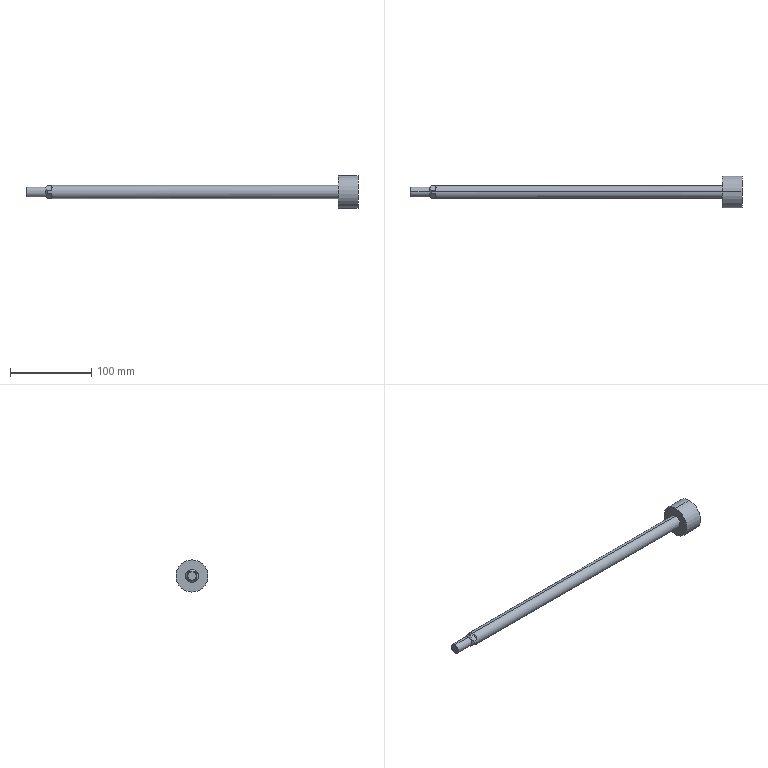Part | SolidWorks | features BaseBody 1 | 1 solid | 21 faces | box 407.5 x 39.5 x 39.5 mm | volume 104182 mm3 | plane 11 | cylinder 6 | cone 4 | commonest cylinder face diameters 12 x2 16 x2 39.5 x2
STEP:
#1=CARTESIAN_POINT('',(334.5,0.,-19.75));
#2=VERTEX_POINT('',#1);
#3=CARTESIAN_POINT('',(358.5,0.,-19.75));
#4=VERTEX_POINT('',#3);
#5=CARTESIAN_POINT('',(358.5,0.,-19.75));
#6=DIRECTION('',(1.,0.,0.));
#7=VECTOR('',#6,1000.);
#8=LINE('',#5,#7);
#9=EDGE_CURVE('',#2,#4,#8,.T.);
#10=ORIENTED_EDGE('',*,*,#9,.F.);
#11=CARTESIAN_POINT('',(334.5,0.,19.75));
#12=VERTEX_POINT('',#11);
#13=CARTESIAN_POINT('',(334.5,0.,0.));
#14=DIRECTION('',(1.,0.,0.));
#15=DIRECTION('',(0.,0.,-1.));
#16=AXIS2_PLACEMENT_3D('',#13,#14,#15);
#17=CIRCLE('',#16,19.75);
#18=EDGE_CURVE('',#2,#12,#17,.T.);
#19=ORIENTED_EDGE('',*,*,#18,.T.);
#20=CARTESIAN_POINT('',(358.5,-0.000000023,19.75));
#21=VERTEX_POINT('',#20);
#22=CARTESIAN_POINT('',(358.5,0.,19.75));
#23=DIRECTION('',(1.,0.,0.));
#24=VECTOR('',#23,1000.);
#25=LINE('',#22,#24);
#26=EDGE_CURVE('',#12,#21,#25,.T.);
#27=ORIENTED_EDGE('',*,*,#26,.T.);
#28=CARTESIAN_POINT('',(358.5,0.,0.));
#29=DIRECTION('',(1.,0.,0.));
#30=DIRECTION('',(0.,-0.000000001,1.));
#31=AXIS2_PLACEMENT_3D('',#28,#29,#30);
#32=CIRCLE('',#31,19.75);
#33=EDGE_CURVE('',#4,#21,#32,.T.);
#34=ORIENTED_EDGE('',*,*,#33,.F.);
#35=EDGE_LOOP('',(#10,#19,#27,#34));
#36=FACE_OUTER_BOUND('',#35,.T.);
#37=CARTESIAN_POINT('',(358.5,0.,0.));
#38=DIRECTION('',(1.,0.,0.));
#39=DIRECTION('',(0.,0.,1.));
#40=AXIS2_PLACEMENT_3D('',#37,#38,#39);
#41=CYLINDRICAL_SURFACE('',#40,19.75);
#42=ADVANCED_FACE('',(#36),#41,.T.);
#43=CARTESIAN_POINT('',(-48.233,0.,-6.));
#44=VERTEX_POINT('',#43);
#45=CARTESIAN_POINT('',(-25.,0.,-6.));
#46=VERTEX_POINT('',#45);
#47=CARTESIAN_POINT('',(358.5,0.,-6.));
#48=DIRECTION('',(1.,0.,0.));
#49=VECTOR('',#48,1000.);
#50=LINE('',#47,#49);
#51=EDGE_CURVE('',#44,#46,#50,.T.);
#52=ORIENTED_EDGE('',*,*,#51,.F.);
#53=CARTESIAN_POINT('',(-48.233,0.,6.));
#54=VERTEX_POINT('',#53);
#55=CARTESIAN_POINT('',(-48.233,0.,0.));
#56=DIRECTION('',(1.,0.,0.));
#57=DIRECTION('',(0.,0.,-1.));
#58=AXIS2_PLACEMENT_3D('',#55,#56,#57);
#59=CIRCLE('',#58,6.);
#60=EDGE_CURVE('',#44,#54,#59,.T.);
#61=ORIENTED_EDGE('',*,*,#60,.T.);
#62=CARTESIAN_POINT('',(-25.,0.,6.));
#63=VERTEX_POINT('',#62);
#64=CARTESIAN_POINT('',(358.5,0.,6.));
#65=DIRECTION('',(1.,0.,0.));
#66=VECTOR('',#65,1000.);
#67=LINE('',#64,#66);
#68=EDGE_CURVE('',#54,#63,#67,.T.);
#69=ORIENTED_EDGE('',*,*,#68,.T.);
#70=CARTESIAN_POINT('',(-25.,0.,0.));
#71=DIRECTION('',(1.,0.,0.));
#72=DIRECTION('',(0.,0.,1.));
#73=AXIS2_PLACEMENT_3D('',#70,#71,#72);
#74=CIRCLE('',#73,6.);
#75=EDGE_CURVE('',#46,#63,#74,.T.);
#76=ORIENTED_EDGE('',*,*,#75,.F.);
#77=EDGE_LOOP('',(#52,#61,#69,#76));
#78=FACE_OUTER_BOUND('',#77,.T.);
#79=CARTESIAN_POINT('',(358.5,0.,0.));
#80=DIRECTION('',(1.,0.,0.));
#81=DIRECTION('',(0.,0.,1.));
#82=AXIS2_PLACEMENT_3D('',#79,#80,#81);
#83=CYLINDRICAL_SURFACE('',#82,6.);
#84=ADVANCED_FACE('',(#78),#83,.T.);
#85=CARTESIAN_POINT('',(-49.,0.,-5.233));
#86=VERTEX_POINT('',#85);
#87=CARTESIAN_POINT('',(-48.233,0.,-6.));
#88=DIRECTION('',(0.7071,0.,-0.7071));
#89=VECTOR('',#88,1000.);
#90=LINE('',#87,#89);
#91=EDGE_CURVE('',#86,#44,#90,.T.);
#92=ORIENTED_EDGE('',*,*,#91,.F.);
#93=CARTESIAN_POINT('',(-49.,0.,5.233));
#94=VERTEX_POINT('',#93);
#95=CARTESIAN_POINT('',(-49.,0.,0.));
#96=DIRECTION('',(1.,0.,0.));
#97=DIRECTION('',(0.,0.,-1.));
#98=AXIS2_PLACEMENT_3D('',#95,#96,#97);
#99=CIRCLE('',#98,5.233);
#100=EDGE_CURVE('',#86,#94,#99,.T.);
#101=ORIENTED_EDGE('',*,*,#100,.T.);
#102=CARTESIAN_POINT('',(-48.233,0.,6.));
#103=DIRECTION('',(0.7071,0.,0.7071));
#104=VECTOR('',#103,1000.);
#105=LINE('',#102,#104);
#106=EDGE_CURVE('',#94,#54,#105,.T.);
#107=ORIENTED_EDGE('',*,*,#106,.T.);
#108=ORIENTED_EDGE('',*,*,#60,.F.);
#109=EDGE_LOOP('',(#92,#101,#107,#108));
#110=FACE_OUTER_BOUND('',#109,.T.);
#111=CARTESIAN_POINT('',(-48.233,0.,0.));
#112=DIRECTION('',(1.,0.,0.));
#113=DIRECTION('',(0.,0.,1.));
#114=AXIS2_PLACEMENT_3D('',#111,#112,#113);
#115=CONICAL_SURFACE('',#114,6.,0.7854);
#116=ADVANCED_FACE('',(#110),#115,.T.);
#117=CARTESIAN_POINT('',(-23.,0.,-8.));
#118=VERTEX_POINT('',#117);
#119=CARTESIAN_POINT('',(334.5,0.,-8.));
#120=VERTEX_POINT('',#119);
#121=CARTESIAN_POINT('',(358.5,0.,-8.));
#122=DIRECTION('',(1.,0.,0.));
#123=VECTOR('',#122,1000.);
#124=LINE('',#121,#123);
#125=EDGE_CURVE('',#118,#120,#124,.T.);
#126=ORIENTED_EDGE('',*,*,#125,.F.);
#127=CARTESIAN_POINT('',(-23.,2.211,-7.688));
#128=VERTEX_POINT('',#127);
#129=CARTESIAN_POINT('',(-23.,0.,0.));
#130=DIRECTION('',(1.,0.,0.));
#131=DIRECTION('',(0.,0.2764,-0.961));
#132=AXIS2_PLACEMENT_3D('',#129,#130,#131);
#133=CIRCLE('',#132,8.);
#134=EDGE_CURVE('',#118,#128,#133,.T.);
#135=ORIENTED_EDGE('',*,*,#134,.T.);
#136=CARTESIAN_POINT('',(-18.,2.211,-7.688));
#137=VERTEX_POINT('',#136);
#138=CARTESIAN_POINT('',(-18.,2.211,-7.688));
#139=DIRECTION('',(-1.,0.,0.));
#140=VECTOR('',#139,1000.);
#141=LINE('',#138,#140);
#142=EDGE_CURVE('',#137,#128,#141,.T.);
#143=ORIENTED_EDGE('',*,*,#142,.F.);
#144=CARTESIAN_POINT('',(-18.,7.688,-2.211));
#145=VERTEX_POINT('',#144);
#146=CARTESIAN_POINT('',(-18.,7.688,-2.211));
#147=CARTESIAN_POINT('',(-17.344,7.314,-3.513));
#148=CARTESIAN_POINT('',(-17.,6.615,-4.699));
#149=CARTESIAN_POINT('',(-17.,4.699,-6.615));
#150=CARTESIAN_POINT('',(-17.344,3.513,-7.314));
#151=CARTESIAN_POINT('',(-18.,2.211,-7.688));
#152=B_SPLINE_CURVE_WITH_KNOTS('',3,(#146,#147,#148,#149,#150,#151),.UNSPECIFIED.,.F.,.F.,(4,2,4),(0.,0.5,1.),.UNSPECIFIED.);
#153=EDGE_CURVE('',#145,#137,#152,.T.);
#154=ORIENTED_EDGE('',*,*,#153,.F.);
#155=CARTESIAN_POINT('',(-23.,7.688,-2.211));
#156=VERTEX_POINT('',#155);
#157=CARTESIAN_POINT('',(-23.,7.688,-2.211));
#158=DIRECTION('',(1.,0.,0.));
#159=VECTOR('',#158,1000.);
#160=LINE('',#157,#159);
#161=EDGE_CURVE('',#156,#145,#160,.T.);
#162=ORIENTED_EDGE('',*,*,#161,.F.);
#163=CARTESIAN_POINT('',(-23.,7.688,2.211));
#164=VERTEX_POINT('',#163);
#165=CARTESIAN_POINT('',(-23.,0.,0.));
#166=DIRECTION('',(1.,0.,0.));
#167=DIRECTION('',(0.,0.961,0.2764));
#168=AXIS2_PLACEMENT_3D('',#165,#166,#167);
#169=CIRCLE('',#168,8.);
#170=EDGE_CURVE('',#156,#164,#169,.T.);
#171=ORIENTED_EDGE('',*,*,#170,.T.);
#172=CARTESIAN_POINT('',(-18.,7.688,2.211));
#173=VERTEX_POINT('',#172);
#174=CARTESIAN_POINT('',(-18.,7.688,2.211));
#175=DIRECTION('',(-1.,0.,0.));
#176=VECTOR('',#175,1000.);
#177=LINE('',#174,#176);
#178=EDGE_CURVE('',#173,#164,#177,.T.);
#179=ORIENTED_EDGE('',*,*,#178,.F.);
#180=CARTESIAN_POINT('',(-18.,2.211,7.688));
#181=VERTEX_POINT('',#180);
#182=CARTESIAN_POINT('',(-18.,2.211,7.688));
#183=CARTESIAN_POINT('',(-17.835,2.539,7.594));
#184=CARTESIAN_POINT('',(-17.69,2.858,7.48));
#185=CARTESIAN_POINT('',(-17.44,3.478,7.213));
#186=CARTESIAN_POINT('',(-17.335,3.781,7.058));
#187=CARTESIAN_POINT('',(-17.167,4.365,6.713));
#188=CARTESIAN_POINT('',(-17.072,4.783,6.429));
#189=CARTESIAN_POINT('',(-17.025,5.172,6.106));
#190=CARTESIAN_POINT('',(-17.004,5.425,5.883));
#191=CARTESIAN_POINT('',(-16.999,5.546,5.768));
#192=CARTESIAN_POINT('',(-17.,5.909,5.404));
#193=CARTESIAN_POINT('',(-17.034,6.246,5.02));
#194=CARTESIAN_POINT('',(-17.13,6.594,4.535));
#195=CARTESIAN_POINT('',(-17.193,6.757,4.284));
#196=CARTESIAN_POINT('',(-17.222,6.824,4.175));
#197=CARTESIAN_POINT('',(-17.243,6.869,4.101));
#198=CARTESIAN_POINT('',(-17.254,6.891,4.063));
#199=CARTESIAN_POINT('',(-17.433,7.246,3.455));
#200=CARTESIAN_POINT('',(-17.679,7.505,2.849));
#201=CARTESIAN_POINT('',(-18.,7.688,2.211));
#202=B_SPLINE_CURVE_WITH_KNOTS('',3,(#182,#183,#184,#185,#186,#187,#188,#189,#190,#191,#192,#193,#194,#195,#196,#197,#198,#199,#200,#201),.UNSPECIFIED.,.F.,.F.,(4,2,2,1,2,2,1,1,1,2,2,4),(0.,0.125,0.25,0.375,0.4375,0.5,0.625,0.6875,0.7187,0.7344,0.75,1.),.UNSPECIFIED.);
#203=EDGE_CURVE('',#181,#173,#202,.T.);
#204=ORIENTED_EDGE('',*,*,#203,.F.);
#205=CARTESIAN_POINT('',(-23.,2.211,7.688));
#206=VERTEX_POINT('',#205);
#207=CARTESIAN_POINT('',(-23.,2.211,7.688));
#208=DIRECTION('',(1.,0.,0.));
#209=VECTOR('',#208,1000.);
#210=LINE('',#207,#209);
#211=EDGE_CURVE('',#206,#181,#210,.T.);
#212=ORIENTED_EDGE('',*,*,#211,.F.);
#213=CARTESIAN_POINT('',(-23.,0.,8.));
#214=VERTEX_POINT('',#213);
#215=CARTESIAN_POINT('',(-23.,0.,0.));
#216=DIRECTION('',(1.,0.,0.));
#217=DIRECTION('',(0.,-0.2764,0.961));
#218=AXIS2_PLACEMENT_3D('',#215,#216,#217);
#219=CIRCLE('',#218,8.);
#220=EDGE_CURVE('',#206,#214,#219,.T.);
#221=ORIENTED_EDGE('',*,*,#220,.T.);
#222=CARTESIAN_POINT('',(334.5,0.,8.));
#223=VERTEX_POINT('',#222);
#224=CARTESIAN_POINT('',(358.5,0.,8.));
#225=DIRECTION('',(1.,0.,0.));
#226=VECTOR('',#225,1000.);
#227=LINE('',#224,#226);
#228=EDGE_CURVE('',#214,#223,#227,.T.);
#229=ORIENTED_EDGE('',*,*,#228,.T.);
#230=CARTESIAN_POINT('',(334.5,0.,0.));
#231=DIRECTION('',(1.,0.,0.));
#232=DIRECTION('',(0.,0.,1.));
#233=AXIS2_PLACEMENT_3D('',#230,#231,#232);
#234=CIRCLE('',#233,8.);
#235=EDGE_CURVE('',#120,#223,#234,.T.);
#236=ORIENTED_EDGE('',*,*,#235,.F.);
#237=EDGE_LOOP('',(#126,#135,#143,#154,#162,#171,#179,#204,#212,#221,#229,#236));
#238=FACE_OUTER_BOUND('',#237,.T.);
#239=CARTESIAN_POINT('',(358.5,0.,0.));
#240=DIRECTION('',(1.,0.,0.));
#241=DIRECTION('',(0.,0.,1.));
#242=AXIS2_PLACEMENT_3D('',#239,#240,#241);
#243=CYLINDRICAL_SURFACE('',#242,8.);
#244=ADVANCED_FACE('',(#238),#243,.T.);
#245=CARTESIAN_POINT('',(-23.,0.,-8.));
#246=DIRECTION('',(0.7071,0.,-0.7071));
#247=VECTOR('',#246,1000.);
#248=LINE('',#245,#247);
#249=EDGE_CURVE('',#46,#118,#248,.T.);
#250=ORIENTED_EDGE('',*,*,#249,.F.);
#251=ORIENTED_EDGE('',*,*,#75,.T.);
#252=CARTESIAN_POINT('',(-23.,0.,8.));
#253=DIRECTION('',(0.7071,0.,0.7071));
#254=VECTOR('',#253,1000.);
#255=LINE('',#252,#254);
#256=EDGE_CURVE('',#63,#214,#255,.T.);
#257=ORIENTED_EDGE('',*,*,#256,.T.);
#258=ORIENTED_EDGE('',*,*,#220,.F.);
#259=CARTESIAN_POINT('',(-23.,7.688,2.211));
#260=CARTESIAN_POINT('',(-23.157,7.459,2.44));
#261=CARTESIAN_POINT('',(-23.364,7.123,2.776));
#262=CARTESIAN_POINT('',(-23.556,6.746,3.153));
#263=CARTESIAN_POINT('',(-23.639,6.561,3.338));
#264=CARTESIAN_POINT('',(-23.678,6.47,3.43));
#265=CARTESIAN_POINT('',(-23.696,6.424,3.476));
#266=CARTESIAN_POINT('',(-23.704,6.404,3.495));
#267=CARTESIAN_POINT('',(-23.709,6.391,3.508));
#268=CARTESIAN_POINT('',(-23.712,6.386,3.514));
#269=CARTESIAN_POINT('',(-23.805,6.147,3.753));
#270=CARTESIAN_POINT('',(-23.909,5.802,4.098));
#271=CARTESIAN_POINT('',(-23.973,5.405,4.495));
#272=CARTESIAN_POINT('',(-23.991,5.207,4.692));
#273=CARTESIAN_POINT('',(-23.995,5.123,4.776));
#274=CARTESIAN_POINT('',(-23.998,5.067,4.833));
#275=CARTESIAN_POINT('',(-23.998,5.04,4.859));
#276=CARTESIAN_POINT('',(-24.003,4.777,5.123));
#277=CARTESIAN_POINT('',(-23.974,4.422,5.477));
#278=CARTESIAN_POINT('',(-23.876,4.002,5.897));
#279=CARTESIAN_POINT('',(-23.811,3.791,6.109));
#280=CARTESIAN_POINT('',(-23.775,3.685,6.215));
#281=CARTESIAN_POINT('',(-23.756,3.632,6.268));
#282=CARTESIAN_POINT('',(-23.748,3.609,6.291));
#283=CARTESIAN_POINT('',(-23.742,3.594,6.306));
#284=CARTESIAN_POINT('',(-23.739,3.585,6.314));
#285=CARTESIAN_POINT('',(-23.573,3.145,6.754));
#286=CARTESIAN_POINT('',(-23.327,2.689,7.21));
#287=CARTESIAN_POINT('',(-23.,2.211,7.688));
#288=B_SPLINE_CURVE_WITH_KNOTS('',3,(#259,#260,#261,#262,#263,#264,#265,#266,#267,#268,#269,#270,#271,#272,#273,#274,#275,#276,#277,#278,#279,#280,#281,#282,#283,#284,#285,#286,#287),.UNSPECIFIED.,.F.,.F.,(4,1,1,1,1,1,2,2,1,1,1,2,2,1,1,1,1,1,2,2,4),(0.,0.125,0.1875,0.2188,0.2344,0.2422,0.2461,0.25,0.375,0.4375,0.4687,0.4844,0.5,0.625,0.6875,0.7187,0.7344,0.7422,0.7461,0.75,1.),.UNSPECIFIED.);
#289=EDGE_CURVE('',#164,#206,#288,.T.);
#290=ORIENTED_EDGE('',*,*,#289,.F.);
#291=ORIENTED_EDGE('',*,*,#170,.F.);
#292=CARTESIAN_POINT('',(-23.,2.211,-7.688));
#293=CARTESIAN_POINT('',(-23.157,2.44,-7.459));
#294=CARTESIAN_POINT('',(-23.364,2.776,-7.123));
#295=CARTESIAN_POINT('',(-23.556,3.153,-6.746));
#296=CARTESIAN_POINT('',(-23.639,3.338,-6.561));
#297=CARTESIAN_POINT('',(-23.678,3.43,-6.47));
#298=CARTESIAN_POINT('',(-23.696,3.476,-6.424));
#299=CARTESIAN_POINT('',(-23.704,3.495,-6.404));
#300=CARTESIAN_POINT('',(-23.709,3.508,-6.391));
#301=CARTESIAN_POINT('',(-23.712,3.514,-6.386));
#302=CARTESIAN_POINT('',(-23.805,3.753,-6.147));
#303=CARTESIAN_POINT('',(-23.909,4.098,-5.802));
#304=CARTESIAN_POINT('',(-23.973,4.495,-5.405));
#305=CARTESIAN_POINT('',(-23.991,4.692,-5.207));
#306=CARTESIAN_POINT('',(-23.995,4.776,-5.123));
#307=CARTESIAN_POINT('',(-23.998,4.833,-5.067));
#308=CARTESIAN_POINT('',(-23.998,4.859,-5.04));
#309=CARTESIAN_POINT('',(-24.003,5.123,-4.777));
#310=CARTESIAN_POINT('',(-23.974,5.477,-4.422));
#311=CARTESIAN_POINT('',(-23.876,5.897,-4.002));
#312=CARTESIAN_POINT('',(-23.811,6.109,-3.791));
#313=CARTESIAN_POINT('',(-23.775,6.215,-3.685));
#314=CARTESIAN_POINT('',(-23.756,6.268,-3.632));
#315=CARTESIAN_POINT('',(-23.748,6.291,-3.609));
#316=CARTESIAN_POINT('',(-23.742,6.306,-3.594));
#317=CARTESIAN_POINT('',(-23.739,6.314,-3.585));
#318=CARTESIAN_POINT('',(-23.573,6.754,-3.145));
#319=CARTESIAN_POINT('',(-23.327,7.21,-2.689));
#320=CARTESIAN_POINT('',(-23.,7.688,-2.211));
#321=B_SPLINE_CURVE_WITH_KNOTS('',3,(#292,#293,#294,#295,#296,#297,#298,#299,#300,#301,#302,#303,#304,#305,#306,#307,#308,#309,#310,#311,#312,#313,#314,#315,#316,#317,#318,#319,#320),.UNSPECIFIED.,.F.,.F.,(4,1,1,1,1,1,2,2,1,1,1,2,2,1,1,1,1,1,2,2,4),(0.,0.125,0.1875,0.2188,0.2344,0.2422,0.2461,0.25,0.375,0.4375,0.4688,0.4844,0.5,0.625,0.6875,0.7188,0.7344,0.7422,0.7461,0.75,1.),.UNSPECIFIED.);
#322=EDGE_CURVE('',#128,#156,#321,.T.);
#323=ORIENTED_EDGE('',*,*,#322,.F.);
#324=ORIENTED_EDGE('',*,*,#134,.F.);
#325=EDGE_LOOP('',(#250,#251,#257,#258,#290,#291,#323,#324));
#326=FACE_OUTER_BOUND('',#325,.T.);
#327=CARTESIAN_POINT('',(-23.,0.,0.));
#328=DIRECTION('',(1.,0.,0.));
#329=DIRECTION('',(0.,0.,1.));
#330=AXIS2_PLACEMENT_3D('',#327,#328,#329);
#331=CONICAL_SURFACE('',#330,8.,0.7854);
#332=ADVANCED_FACE('',(#326),#331,.T.);
#333=ORIENTED_EDGE('',*,*,#161,.T.);
#334=CARTESIAN_POINT('',(-18.,2.211,-7.688));
#335=DIRECTION('',(0.,0.7071,0.7071));
#336=VECTOR('',#335,1000.);
#337=LINE('',#334,#336);
#338=EDGE_CURVE('',#137,#145,#337,.T.);
#339=ORIENTED_EDGE('',*,*,#338,.F.);
#340=ORIENTED_EDGE('',*,*,#142,.T.);
#341=ORIENTED_EDGE('',*,*,#322,.T.);
#342=EDGE_LOOP('',(#333,#339,#340,#341));
#343=FACE_OUTER_BOUND('',#342,.T.);
#344=CARTESIAN_POINT('',(-24.151,2.211,-7.688));
#345=DIRECTION('',(0.,0.7071,-0.7071));
#346=DIRECTION('',(-1.,0.,0.));
#347=AXIS2_PLACEMENT_3D('',#344,#345,#346);
#348=PLANE('',#347);
#349=ADVANCED_FACE('',(#343),#348,.T.);
#350=ORIENTED_EDGE('',*,*,#153,.T.);
#351=ORIENTED_EDGE('',*,*,#338,.T.);
#352=EDGE_LOOP('',(#350,#351));
#353=FACE_OUTER_BOUND('',#352,.T.);
#354=CARTESIAN_POINT('',(-17.979,2.211,-7.718));
#355=DIRECTION('',(-0.7071,0.5,-0.5));
#356=DIRECTION('',(-0.5774,0.,0.8165));
#357=AXIS2_PLACEMENT_3D('',#354,#355,#356);
#358=PLANE('',#357);
#359=ADVANCED_FACE('',(#353),#358,.T.);
#360=CARTESIAN_POINT('',(-23.,-7.688,2.211));
#361=VERTEX_POINT('',#360);
#362=CARTESIAN_POINT('',(-18.,-7.688,2.211));
#363=VERTEX_POINT('',#362);
#364=CARTESIAN_POINT('',(-23.,-7.688,2.211));
#365=DIRECTION('',(1.,0.,0.));
#366=VECTOR('',#365,1000.);
#367=LINE('',#364,#366);
#368=EDGE_CURVE('',#361,#363,#367,.T.);
#369=ORIENTED_EDGE('',*,*,#368,.T.);
#370=CARTESIAN_POINT('',(-18.,-2.211,7.688));
#371=VERTEX_POINT('',#370);
#372=CARTESIAN_POINT('',(-18.,-2.211,7.688));
#373=DIRECTION('',(0.,0.7071,0.7071));
#374=VECTOR('',#373,1000.);
#375=LINE('',#372,#374);
#376=EDGE_CURVE('',#363,#371,#375,.T.);
#377=ORIENTED_EDGE('',*,*,#376,.T.);
#378=CARTESIAN_POINT('',(-23.,-2.211,7.688));
#379=VERTEX_POINT('',#378);
#380=CARTESIAN_POINT('',(-18.,-2.211,7.688));
#381=DIRECTION('',(-1.,0.,0.));
#382=VECTOR('',#381,1000.);
#383=LINE('',#380,#382);
#384=EDGE_CURVE('',#371,#379,#383,.T.);
#385=ORIENTED_EDGE('',*,*,#384,.T.);
#386=CARTESIAN_POINT('',(-23.,-2.211,7.688));
#387=CARTESIAN_POINT('',(-23.157,-2.44,7.459));
#388=CARTESIAN_POINT('',(-23.364,-2.776,7.123));
#389=CARTESIAN_POINT('',(-23.556,-3.153,6.746));
#390=CARTESIAN_POINT('',(-23.639,-3.338,6.561));
#391=CARTESIAN_POINT('',(-23.678,-3.43,6.47));
#392=CARTESIAN_POINT('',(-23.696,-3.476,6.424));
#393=CARTESIAN_POINT('',(-23.704,-3.495,6.404));
#394=CARTESIAN_POINT('',(-23.709,-3.508,6.391));
#395=CARTESIAN_POINT('',(-23.712,-3.514,6.386));
#396=CARTESIAN_POINT('',(-23.805,-3.753,6.147));
#397=CARTESIAN_POINT('',(-23.909,-4.098,5.802));
#398=CARTESIAN_POINT('',(-23.973,-4.495,5.405));
#399=CARTESIAN_POINT('',(-23.991,-4.692,5.207));
#400=CARTESIAN_POINT('',(-23.995,-4.776,5.123));
#401=CARTESIAN_POINT('',(-23.998,-4.833,5.067));
#402=CARTESIAN_POINT('',(-23.998,-4.859,5.04));
#403=CARTESIAN_POINT('',(-24.003,-5.123,4.777));
#404=CARTESIAN_POINT('',(-23.974,-5.477,4.422));
#405=CARTESIAN_POINT('',(-23.876,-5.897,4.002));
#406=CARTESIAN_POINT('',(-23.811,-6.109,3.791));
#407=CARTESIAN_POINT('',(-23.775,-6.215,3.685));
#408=CARTESIAN_POINT('',(-23.756,-6.268,3.632));
#409=CARTESIAN_POINT('',(-23.748,-6.291,3.609));
#410=CARTESIAN_POINT('',(-23.742,-6.306,3.594));
#411=CARTESIAN_POINT('',(-23.739,-6.314,3.585));
#412=CARTESIAN_POINT('',(-23.573,-6.754,3.145));
#413=CARTESIAN_POINT('',(-23.327,-7.21,2.689));
#414=CARTESIAN_POINT('',(-23.,-7.688,2.211));
#415=B_SPLINE_CURVE_WITH_KNOTS('',3,(#386,#387,#388,#389,#390,#391,#392,#393,#394,#395,#396,#397,#398,#399,#400,#401,#402,#403,#404,#405,#406,#407,#408,#409,#410,#411,#412,#413,#414),.UNSPECIFIED.,.F.,.F.,(4,1,1,1,1,1,2,2,1,1,1,2,2,1,1,1,1,1,2,2,4),(0.,0.125,0.1875,0.2187,0.2344,0.2422,0.2461,0.25,0.375,0.4375,0.4687,0.4844,0.5,0.625,0.6875,0.7188,0.7344,0.7422,0.7461,0.75,1.),.UNSPECIFIED.);
#416=EDGE_CURVE('',#379,#361,#415,.T.);
#417=ORIENTED_EDGE('',*,*,#416,.T.);
#418=EDGE_LOOP('',(#369,#377,#385,#417));
#419=FACE_OUTER_BOUND('',#418,.T.);
#420=CARTESIAN_POINT('',(-24.151,-2.211,7.688));
#421=DIRECTION('',(0.,-0.7071,0.7071));
#422=DIRECTION('',(-1.,0.,0.));
#423=AXIS2_PLACEMENT_3D('',#420,#421,#422);
#424=PLANE('',#423);
#425=ADVANCED_FACE('',(#419),#424,.T.);
#426=CARTESIAN_POINT('',(-18.,-7.688,2.211));
#427=CARTESIAN_POINT('',(-17.344,-7.314,3.513));
#428=CARTESIAN_POINT('',(-17.,-6.615,4.699));
#429=CARTESIAN_POINT('',(-17.,-4.699,6.615));
#430=CARTESIAN_POINT('',(-17.344,-3.513,7.314));
#431=CARTESIAN_POINT('',(-18.,-2.211,7.688));
#432=B_SPLINE_CURVE_WITH_KNOTS('',3,(#426,#427,#428,#429,#430,#431),.UNSPECIFIED.,.F.,.F.,(4,2,4),(0.,0.5,1.),.UNSPECIFIED.);
#433=EDGE_CURVE('',#363,#371,#432,.T.);
#434=ORIENTED_EDGE('',*,*,#433,.T.);
#435=ORIENTED_EDGE('',*,*,#376,.F.);
#436=EDGE_LOOP('',(#434,#435));
#437=FACE_OUTER_BOUND('',#436,.T.);
#438=CARTESIAN_POINT('',(-18.,-7.688,2.211));
#439=DIRECTION('',(-0.7071,-0.5,0.5));
#440=DIRECTION('',(-0.5774,0.8165,0.));
#441=AXIS2_PLACEMENT_3D('',#438,#439,#440);
#442=PLANE('',#441);
#443=ADVANCED_FACE('',(#437),#442,.T.);
#444=CARTESIAN_POINT('',(-23.,-2.211,-7.688));
#445=VERTEX_POINT('',#444);
#446=CARTESIAN_POINT('',(-18.,-2.211,-7.688));
#447=VERTEX_POINT('',#446);
#448=CARTESIAN_POINT('',(-23.,-2.211,-7.688));
#449=DIRECTION('',(1.,0.,0.));
#450=VECTOR('',#449,1000.);
#451=LINE('',#448,#450);
#452=EDGE_CURVE('',#445,#447,#451,.T.);
#453=ORIENTED_EDGE('',*,*,#452,.T.);
#454=CARTESIAN_POINT('',(-18.,-7.688,-2.211));
#455=VERTEX_POINT('',#454);
#456=CARTESIAN_POINT('',(-18.,-7.688,-2.211));
#457=DIRECTION('',(0.,0.7071,-0.7071));
#458=VECTOR('',#457,1000.);
#459=LINE('',#456,#458);
#460=EDGE_CURVE('',#455,#447,#459,.T.);
#461=ORIENTED_EDGE('',*,*,#460,.F.);
#462=CARTESIAN_POINT('',(-23.,-7.688,-2.211));
#463=VERTEX_POINT('',#462);
#464=CARTESIAN_POINT('',(-18.,-7.688,-2.211));
#465=DIRECTION('',(-1.,0.,0.));
#466=VECTOR('',#465,1000.);
#467=LINE('',#464,#466);
#468=EDGE_CURVE('',#455,#463,#467,.T.);
#469=ORIENTED_EDGE('',*,*,#468,.T.);
#470=CARTESIAN_POINT('',(-23.,-7.688,-2.211));
#471=CARTESIAN_POINT('',(-23.157,-7.459,-2.44));
#472=CARTESIAN_POINT('',(-23.364,-7.123,-2.776));
#473=CARTESIAN_POINT('',(-23.556,-6.746,-3.153));
#474=CARTESIAN_POINT('',(-23.639,-6.561,-3.338));
#475=CARTESIAN_POINT('',(-23.678,-6.47,-3.43));
#476=CARTESIAN_POINT('',(-23.696,-6.424,-3.476));
#477=CARTESIAN_POINT('',(-23.704,-6.404,-3.495));
#478=CARTESIAN_POINT('',(-23.709,-6.391,-3.508));
#479=CARTESIAN_POINT('',(-23.712,-6.386,-3.514));
#480=CARTESIAN_POINT('',(-23.805,-6.147,-3.753));
#481=CARTESIAN_POINT('',(-23.909,-5.802,-4.098));
#482=CARTESIAN_POINT('',(-23.973,-5.405,-4.495));
#483=CARTESIAN_POINT('',(-23.991,-5.207,-4.692));
#484=CARTESIAN_POINT('',(-23.995,-5.123,-4.776));
#485=CARTESIAN_POINT('',(-23.998,-5.067,-4.833));
#486=CARTESIAN_POINT('',(-23.998,-5.04,-4.859));
#487=CARTESIAN_POINT('',(-24.003,-4.777,-5.123));
#488=CARTESIAN_POINT('',(-23.974,-4.422,-5.477));
#489=CARTESIAN_POINT('',(-23.876,-4.002,-5.897));
#490=CARTESIAN_POINT('',(-23.811,-3.791,-6.109));
#491=CARTESIAN_POINT('',(-23.775,-3.685,-6.215));
#492=CARTESIAN_POINT('',(-23.756,-3.632,-6.268));
#493=CARTESIAN_POINT('',(-23.748,-3.609,-6.291));
#494=CARTESIAN_POINT('',(-23.742,-3.594,-6.306));
#495=CARTESIAN_POINT('',(-23.739,-3.585,-6.314));
#496=CARTESIAN_POINT('',(-23.573,-3.145,-6.754));
#497=CARTESIAN_POINT('',(-23.327,-2.689,-7.21));
#498=CARTESIAN_POINT('',(-23.,-2.211,-7.688));
#499=B_SPLINE_CURVE_WITH_KNOTS('',3,(#470,#471,#472,#473,#474,#475,#476,#477,#478,#479,#480,#481,#482,#483,#484,#485,#486,#487,#488,#489,#490,#491,#492,#493,#494,#495,#496,#497,#498),.UNSPECIFIED.,.F.,.F.,(4,1,1,1,1,1,2,2,1,1,1,2,2,1,1,1,1,1,2,2,4),(0.,0.125,0.1875,0.2188,0.2344,0.2422,0.2461,0.25,0.375,0.4375,0.4688,0.4844,0.5,0.625,0.6875,0.7188,0.7344,0.7422,0.7461,0.75,1.),.UNSPECIFIED.);
#500=EDGE_CURVE('',#463,#445,#499,.T.);
#501=ORIENTED_EDGE('',*,*,#500,.T.);
#502=EDGE_LOOP('',(#453,#461,#469,#501));
#503=FACE_OUTER_BOUND('',#502,.T.);
#504=CARTESIAN_POINT('',(-24.151,-7.688,-2.211));
#505=DIRECTION('',(0.,-0.7071,-0.7071));
#506=DIRECTION('',(0.,-0.7071,0.7071));
#507=AXIS2_PLACEMENT_3D('',#504,#505,#506);
#508=PLANE('',#507);
#509=ADVANCED_FACE('',(#503),#508,.T.);
#510=CARTESIAN_POINT('',(-18.,-2.211,-7.688));
#511=CARTESIAN_POINT('',(-17.835,-2.539,-7.594));
#512=CARTESIAN_POINT('',(-17.69,-2.858,-7.48));
#513=CARTESIAN_POINT('',(-17.44,-3.478,-7.213));
#514=CARTESIAN_POINT('',(-17.335,-3.781,-7.058));
#515=CARTESIAN_POINT('',(-17.167,-4.365,-6.713));
#516=CARTESIAN_POINT('',(-17.072,-4.783,-6.429));
#517=CARTESIAN_POINT('',(-17.025,-5.172,-6.106));
#518=CARTESIAN_POINT('',(-17.004,-5.425,-5.883));
#519=CARTESIAN_POINT('',(-16.999,-5.546,-5.768));
#520=CARTESIAN_POINT('',(-17.,-5.909,-5.404));
#521=CARTESIAN_POINT('',(-17.034,-6.246,-5.02));
#522=CARTESIAN_POINT('',(-17.13,-6.594,-4.535));
#523=CARTESIAN_POINT('',(-17.193,-6.757,-4.284));
#524=CARTESIAN_POINT('',(-17.222,-6.824,-4.175));
#525=CARTESIAN_POINT('',(-17.243,-6.869,-4.101));
#526=CARTESIAN_POINT('',(-17.254,-6.891,-4.063));
#527=CARTESIAN_POINT('',(-17.433,-7.246,-3.455));
#528=CARTESIAN_POINT('',(-17.679,-7.505,-2.849));
#529=CARTESIAN_POINT('',(-18.,-7.688,-2.211));
#530=B_SPLINE_CURVE_WITH_KNOTS('',3,(#510,#511,#512,#513,#514,#515,#516,#517,#518,#519,#520,#521,#522,#523,#524,#525,#526,#527,#528,#529),.UNSPECIFIED.,.F.,.F.,(4,2,2,1,2,2,1,1,1,2,2,4),(0.,0.125,0.25,0.375,0.4375,0.5,0.625,0.6875,0.7188,0.7344,0.75,1.),.UNSPECIFIED.);
#531=EDGE_CURVE('',#447,#455,#530,.T.);
#532=ORIENTED_EDGE('',*,*,#531,.T.);
#533=ORIENTED_EDGE('',*,*,#460,.T.);
#534=EDGE_LOOP('',(#532,#533));
#535=FACE_OUTER_BOUND('',#534,.T.);
#536=CARTESIAN_POINT('',(-15.386,-7.688,-5.907));
#537=DIRECTION('',(-0.7071,-0.5,-0.5));
#538=DIRECTION('',(-0.5774,0.8165,0.));
#539=AXIS2_PLACEMENT_3D('',#536,#537,#538);
#540=PLANE('',#539);
#541=ADVANCED_FACE('',(#535),#540,.T.);
#542=ORIENTED_EDGE('',*,*,#211,.T.);
#543=CARTESIAN_POINT('',(-18.,7.688,2.211));
#544=DIRECTION('',(0.,0.7071,-0.7071));
#545=VECTOR('',#544,1000.);
#546=LINE('',#543,#545);
#547=EDGE_CURVE('',#181,#173,#546,.T.);
#548=ORIENTED_EDGE('',*,*,#547,.T.);
#549=ORIENTED_EDGE('',*,*,#178,.T.);
#550=ORIENTED_EDGE('',*,*,#289,.T.);
#551=EDGE_LOOP('',(#542,#548,#549,#550));
#552=FACE_OUTER_BOUND('',#551,.T.);
#553=CARTESIAN_POINT('',(-24.151,7.688,2.211));
#554=DIRECTION('',(0.,0.7071,0.7071));
#555=DIRECTION('',(1.,0.,0.));
#556=AXIS2_PLACEMENT_3D('',#553,#554,#555);
#557=PLANE('',#556);
#558=ADVANCED_FACE('',(#552),#557,.T.);
#559=ORIENTED_EDGE('',*,*,#203,.T.);
#560=ORIENTED_EDGE('',*,*,#547,.F.);
#561=EDGE_LOOP('',(#559,#560));
#562=FACE_OUTER_BOUND('',#561,.T.);
#563=CARTESIAN_POINT('',(-20.582,2.211,4.037));
#564=DIRECTION('',(-0.7071,0.5,0.5));
#565=DIRECTION('',(0.5774,0.,0.8165));
#566=AXIS2_PLACEMENT_3D('',#563,#564,#565);
#567=PLANE('',#566);
#568=ADVANCED_FACE('',(#562),#567,.T.);
#569=CARTESIAN_POINT('',(358.5,0.,0.));
#570=DIRECTION('',(1.,0.,0.));
#571=DIRECTION('',(0.,-0.000000001,1.));
#572=AXIS2_PLACEMENT_3D('',#569,#570,#571);
#573=CIRCLE('',#572,19.75);
#574=EDGE_CURVE('',#21,#4,#573,.T.);
#575=ORIENTED_EDGE('',*,*,#574,.T.);
#576=ORIENTED_EDGE('',*,*,#33,.T.);
#577=EDGE_LOOP('',(#575,#576));
#578=FACE_OUTER_BOUND('',#577,.T.);
#579=CARTESIAN_POINT('',(358.5,-20.117,-19.75));
#580=DIRECTION('',(1.,0.,0.));
#581=DIRECTION('',(0.,1.,0.));
#582=AXIS2_PLACEMENT_3D('',#579,#580,#581);
#583=PLANE('',#582);
#584=ADVANCED_FACE('',(#578),#583,.T.);
#585=CARTESIAN_POINT('',(334.5,0.,0.));
#586=DIRECTION('',(1.,0.,0.));
#587=DIRECTION('',(0.,0.,1.));
#588=AXIS2_PLACEMENT_3D('',#585,#586,#587);
#589=CIRCLE('',#588,8.);
#590=EDGE_CURVE('',#223,#120,#589,.T.);
#591=ORIENTED_EDGE('',*,*,#590,.T.);
#592=ORIENTED_EDGE('',*,*,#235,.T.);
#593=EDGE_LOOP('',(#591,#592));
#594=FACE_BOUND('',#593,.T.);
#595=CARTESIAN_POINT('',(334.5,0.,0.));
#596=DIRECTION('',(1.,0.,0.));
#597=DIRECTION('',(0.,0.,-1.));
#598=AXIS2_PLACEMENT_3D('',#595,#596,#597);
#599=CIRCLE('',#598,19.75);
#600=EDGE_CURVE('',#12,#2,#599,.T.);
#601=ORIENTED_EDGE('',*,*,#600,.F.);
#602=ORIENTED_EDGE('',*,*,#18,.F.);
#603=EDGE_LOOP('',(#601,#602));
#604=FACE_OUTER_BOUND('',#603,.T.);
#605=CARTESIAN_POINT('',(334.5,-20.117,19.75));
#606=DIRECTION('',(-1.,0.,0.));
#607=DIRECTION('',(0.,0.,1.));
#608=AXIS2_PLACEMENT_3D('',#605,#606,#607);
#609=PLANE('',#608);
#610=ADVANCED_FACE('',(#594,#604),#609,.T.);
#611=CARTESIAN_POINT('',(-49.,0.,0.));
#612=DIRECTION('',(1.,0.,0.));
#613=DIRECTION('',(0.,0.,-1.));
#614=AXIS2_PLACEMENT_3D('',#611,#612,#613);
#615=CIRCLE('',#614,5.233);
#616=EDGE_CURVE('',#94,#86,#615,.T.);
#617=ORIENTED_EDGE('',*,*,#616,.F.);
#618=ORIENTED_EDGE('',*,*,#100,.F.);
#619=EDGE_LOOP('',(#617,#618));
#620=FACE_OUTER_BOUND('',#619,.T.);
#621=CARTESIAN_POINT('',(-49.,-5.304,5.233));
#622=DIRECTION('',(-1.,0.,0.));
#623=DIRECTION('',(0.,0.,1.));
#624=AXIS2_PLACEMENT_3D('',#621,#622,#623);
#625=PLANE('',#624);
#626=ADVANCED_FACE('',(#620),#625,.T.);
#627=CARTESIAN_POINT('',(-25.,0.,0.));
#628=DIRECTION('',(1.,0.,0.));
#629=DIRECTION('',(0.,0.,1.));
#630=AXIS2_PLACEMENT_3D('',#627,#628,#629);
#631=CIRCLE('',#630,6.);
#632=EDGE_CURVE('',#63,#46,#631,.T.);
#633=ORIENTED_EDGE('',*,*,#632,.T.);
#634=ORIENTED_EDGE('',*,*,#249,.T.);
#635=CARTESIAN_POINT('',(-23.,0.,0.));
#636=DIRECTION('',(1.,0.,0.));
#637=DIRECTION('',(0.,0.2764,-0.961));
#638=AXIS2_PLACEMENT_3D('',#635,#636,#637);
#639=CIRCLE('',#638,8.);
#640=EDGE_CURVE('',#445,#118,#639,.T.);
#641=ORIENTED_EDGE('',*,*,#640,.F.);
#642=ORIENTED_EDGE('',*,*,#500,.F.);
#643=CARTESIAN_POINT('',(-23.,0.,0.));
#644=DIRECTION('',(1.,0.,0.));
#645=DIRECTION('',(0.,-0.961,-0.2764));
#646=AXIS2_PLACEMENT_3D('',#643,#644,#645);
#647=CIRCLE('',#646,8.);
#648=EDGE_CURVE('',#361,#463,#647,.T.);
#649=ORIENTED_EDGE('',*,*,#648,.F.);
#650=ORIENTED_EDGE('',*,*,#416,.F.);
#651=CARTESIAN_POINT('',(-23.,0.,0.));
#652=DIRECTION('',(1.,0.,0.));
#653=DIRECTION('',(0.,-0.2764,0.961));
#654=AXIS2_PLACEMENT_3D('',#651,#652,#653);
#655=CIRCLE('',#654,8.);
#656=EDGE_CURVE('',#214,#379,#655,.T.);
#657=ORIENTED_EDGE('',*,*,#656,.F.);
#658=ORIENTED_EDGE('',*,*,#256,.F.);
#659=EDGE_LOOP('',(#633,#634,#641,#642,#649,#650,#657,#658));
#660=FACE_OUTER_BOUND('',#659,.T.);
#661=CARTESIAN_POINT('',(-23.,0.,0.));
#662=DIRECTION('',(1.,0.,0.));
#663=DIRECTION('',(0.,0.,1.));
#664=AXIS2_PLACEMENT_3D('',#661,#662,#663);
#665=CONICAL_SURFACE('',#664,8.,0.7854);
#666=ADVANCED_FACE('',(#660),#665,.T.);
#667=ORIENTED_EDGE('',*,*,#640,.T.);
#668=ORIENTED_EDGE('',*,*,#125,.T.);
#669=ORIENTED_EDGE('',*,*,#590,.F.);
#670=ORIENTED_EDGE('',*,*,#228,.F.);
#671=ORIENTED_EDGE('',*,*,#656,.T.);
#672=ORIENTED_EDGE('',*,*,#384,.F.);
#673=ORIENTED_EDGE('',*,*,#433,.F.);
#674=ORIENTED_EDGE('',*,*,#368,.F.);
#675=ORIENTED_EDGE('',*,*,#648,.T.);
#676=ORIENTED_EDGE('',*,*,#468,.F.);
#677=ORIENTED_EDGE('',*,*,#531,.F.);
#678=ORIENTED_EDGE('',*,*,#452,.F.);
#679=EDGE_LOOP('',(#667,#668,#669,#670,#671,#672,#673,#674,#675,#676,#677,#678));
#680=FACE_OUTER_BOUND('',#679,.T.);
#681=CARTESIAN_POINT('',(358.5,0.,0.));
#682=DIRECTION('',(1.,0.,0.));
#683=DIRECTION('',(0.,0.,1.));
#684=AXIS2_PLACEMENT_3D('',#681,#682,#683);
#685=CYLINDRICAL_SURFACE('',#684,8.);
#686=ADVANCED_FACE('',(#680),#685,.T.);
#687=ORIENTED_EDGE('',*,*,#616,.T.);
#688=ORIENTED_EDGE('',*,*,#91,.T.);
#689=CARTESIAN_POINT('',(-48.233,0.,0.));
#690=DIRECTION('',(1.,0.,0.));
#691=DIRECTION('',(0.,0.,-1.));
#692=AXIS2_PLACEMENT_3D('',#689,#690,#691);
#693=CIRCLE('',#692,6.);
#694=EDGE_CURVE('',#54,#44,#693,.T.);
#695=ORIENTED_EDGE('',*,*,#694,.F.);
#696=ORIENTED_EDGE('',*,*,#106,.F.);
#697=EDGE_LOOP('',(#687,#688,#695,#696));
#698=FACE_OUTER_BOUND('',#697,.T.);
#699=CARTESIAN_POINT('',(-48.233,0.,0.));
#700=DIRECTION('',(1.,0.,0.));
#701=DIRECTION('',(0.,0.,1.));
#702=AXIS2_PLACEMENT_3D('',#699,#700,#701);
#703=CONICAL_SURFACE('',#702,6.,0.7854);
#704=ADVANCED_FACE('',(#698),#703,.T.);
#705=ORIENTED_EDGE('',*,*,#694,.T.);
#706=ORIENTED_EDGE('',*,*,#51,.T.);
#707=ORIENTED_EDGE('',*,*,#632,.F.);
#708=ORIENTED_EDGE('',*,*,#68,.F.);
#709=EDGE_LOOP('',(#705,#706,#707,#708));
#710=FACE_OUTER_BOUND('',#709,.T.);
#711=CARTESIAN_POINT('',(358.5,0.,0.));
#712=DIRECTION('',(1.,0.,0.));
#713=DIRECTION('',(0.,0.,1.));
#714=AXIS2_PLACEMENT_3D('',#711,#712,#713);
#715=CYLINDRICAL_SURFACE('',#714,6.);
#716=ADVANCED_FACE('',(#710),#715,.T.);
#717=ORIENTED_EDGE('',*,*,#600,.T.);
#718=ORIENTED_EDGE('',*,*,#9,.T.);
#719=ORIENTED_EDGE('',*,*,#574,.F.);
#720=ORIENTED_EDGE('',*,*,#26,.F.);
#721=EDGE_LOOP('',(#717,#718,#719,#720));
#722=FACE_OUTER_BOUND('',#721,.T.);
#723=CARTESIAN_POINT('',(358.5,0.,0.));
#724=DIRECTION('',(1.,0.,0.));
#725=DIRECTION('',(0.,0.,1.));
#726=AXIS2_PLACEMENT_3D('',#723,#724,#725);
#727=CYLINDRICAL_SURFACE('',#726,19.75);
#728=ADVANCED_FACE('',(#722),#727,.T.);
#729=CLOSED_SHELL('',(#42,#84,#116,#244,#332,#349,#359,#425,#443,#509,#541,#558,#568,#584,#610,#626,#666,#686,#704,#716,#728));
#730=MANIFOLD_SOLID_BREP('',#729);
#731=CARTESIAN_POINT('',(0.,0.,0.));
#732=DIRECTION('',(0.,0.,1.));
#733=DIRECTION('',(1.,0.,0.));
#734=AXIS2_PLACEMENT_3D('',#731,#732,#733);
#735=(LENGTH_UNIT()NAMED_UNIT(*)SI_UNIT(.MILLI.,.METRE.));
#736=UNCERTAINTY_MEASURE_WITH_UNIT(LENGTH_MEASURE(0.00001),#735,'','');
#737=(NAMED_UNIT(*)PLANE_ANGLE_UNIT()SI_UNIT($,.RADIAN.));
#738=(NAMED_UNIT(*)SI_UNIT($,.STERADIAN.)SOLID_ANGLE_UNIT());
#739=(GEOMETRIC_REPRESENTATION_CONTEXT(3)GLOBAL_UNCERTAINTY_ASSIGNED_CONTEXT((#736))GLOBAL_UNIT_ASSIGNED_CONTEXT((#735,#737,#738))REPRESENTATION_CONTEXT('',''));
#740=ADVANCED_BREP_SHAPE_REPRESENTATION('',(#730,#734),#739);